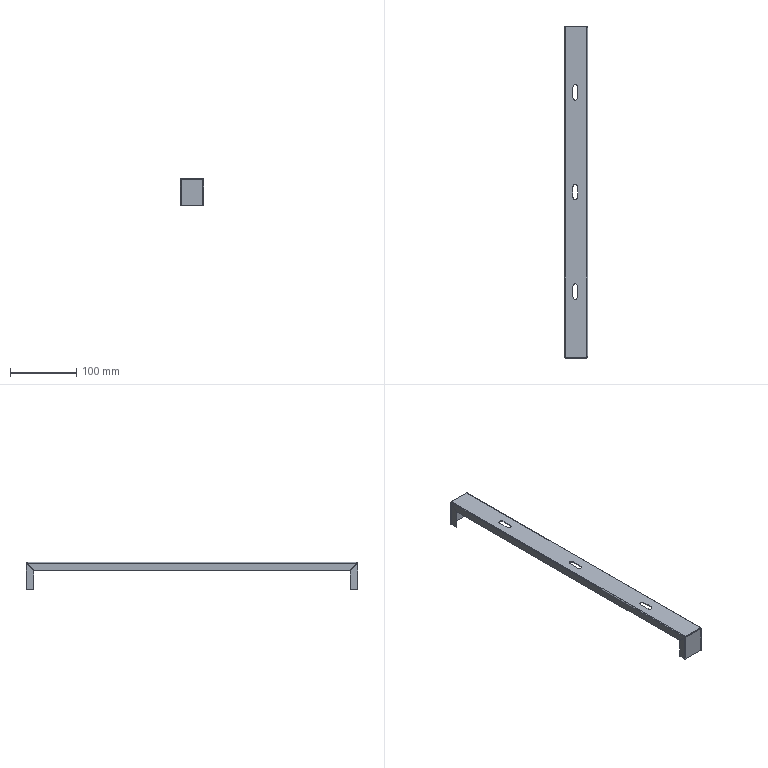Part | SolidWorks | features EdgeFlange 3, FlatPattern 1, SMBaseFlange 1, SheetMetal 1 | 1 solid | 82 faces | box 35 x 500 x 41 mm | volume 37614 mm3 | plane 52 | cylinder 22 | spline 8 | commonest cylinder face diameters 0.4 x8 2.8 x8 7 x6